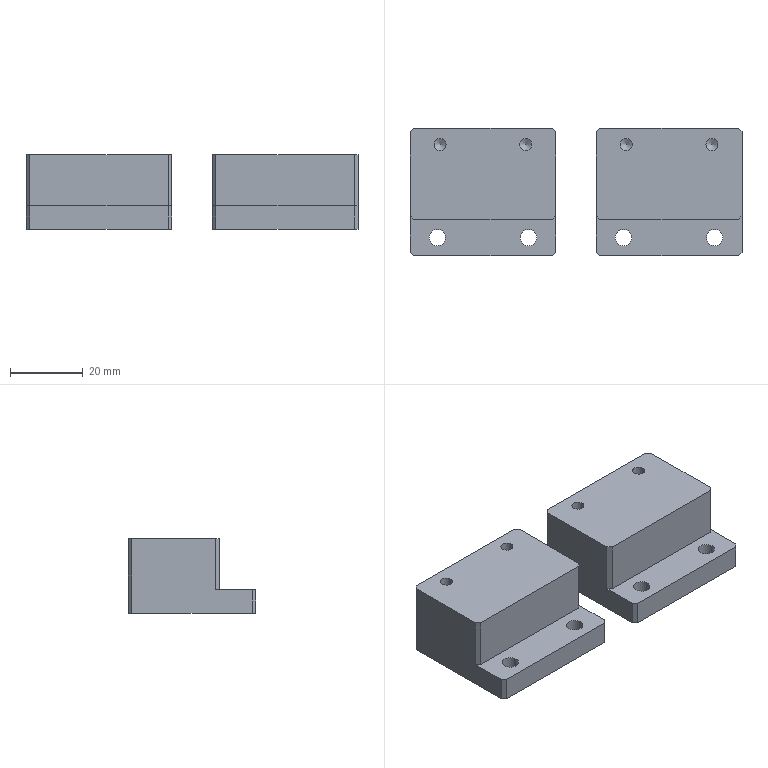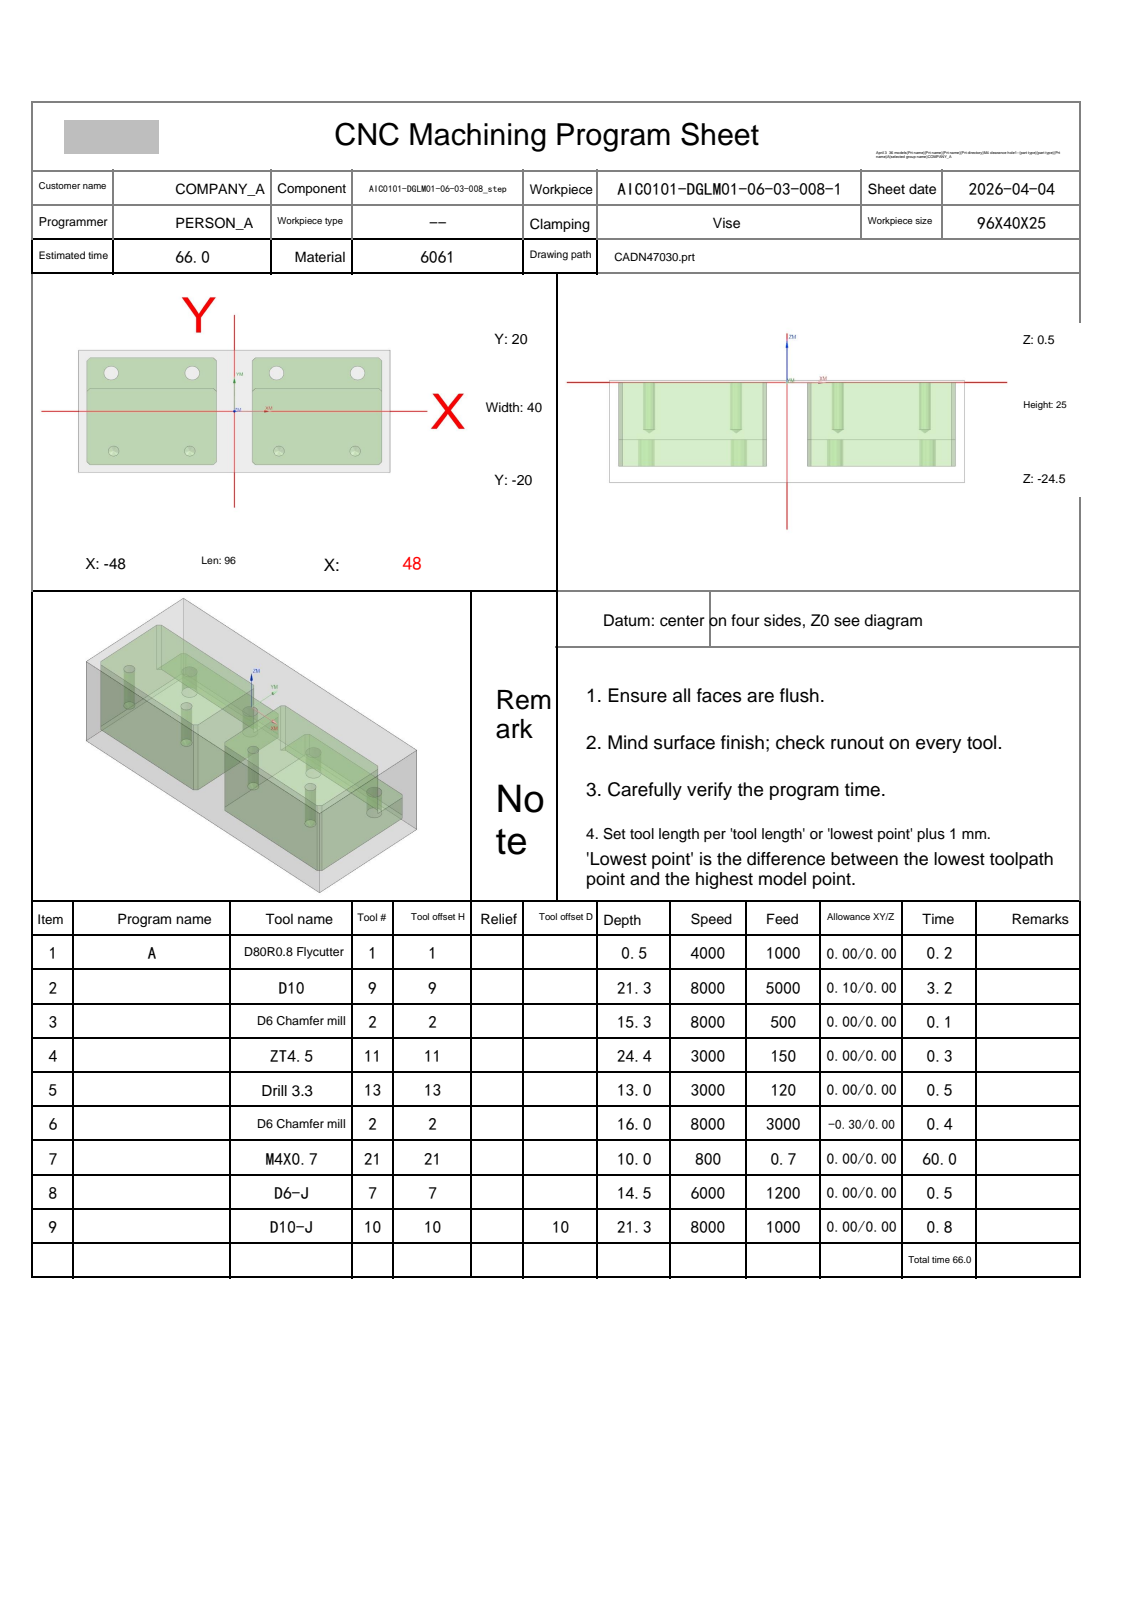NC program | NX | posted by the shop | part box 91 x 35 x 20.5 mm
Lines 1 to 2027 of 2147, first 1232 of 2025 lines:
%
O0001
(Machine time: 121.97 MIN)
(===Total Tool:8===)
(T1=D80R0.8 Flycutter D=80.  R=0.8  D-  H01 Z=-0.   )
(T9=D10     D=10.  R=0.   D-  H09 Z=-20.8 )
(T2=D6 Chamfer mill   D=6.   R=0.   D-  H02 Z=-15.5 )
(T11=ZT4.5  D=4.5  DR_a=118 D-  H11 Z=-23.85)
(T13=Drill 3.3  D=3.3  DR_a=118 D-  H13 Z=-12.49)
(T21=M4X0.7 D=3.3  DR_a=180 D-  H21 Z=-9.5  )
(T7=D6-J    D=6.   R=0.   D7  H07 Z=-14.  )
(T10=D10-J  D=10.  R=0.   D10 H10 Z=-20.8 )
G80 G90 G17 G49 G40
G91 G28 Z0
M01
N1 T01 M06
(D80R0.8 Flycutter  D=80. R=0.8 H=01 ce=0.00 di=0.00)
G00 G90 G54 X90.5 Y0.0 M03 S4000
G43 H01 Z20.
M08
Z2.
G01 Z0.0 F1000.
X85.5
X-85.5
X-90.5
Z2.
G00 Z20.
G91 G28 Z0.0
M05
M09
G91 G28 Z0.0
M01
N2 T09 M06
(D10  D=10. R=0. H=09 ce=0.10 di=0.00)
G00 G90 G54 X25.5 Y-22.6 M03 S8000
G43 H09 Z20.
M08
Z.5
G01 X6.5 Z.417 F5000.
G02 X2.894 Y-21.106 Z.399 I0.0 J5.1
G01 X1.894 Y-20.106 Z.393
G02 X.4 Y-16.5 Z.375 I3.606 J3.606
G01 Y16.5 Z.23
G02 X1.894 Y20.106 Z.213 I5.1 J0.0
G01 X2.894 Y21.106 Z.207
G02 X6.5 Y22.6 Z.189 I3.606 J-3.606
G01 X44.5 Z.022
G02 X48.106 Y21.106 Z.005 I0.0 J-5.1
G01 X49.106 Y20.106 Z-.002
G02 X50.6 Y16.5 Z-.019 I-3.606 J-3.606
G01 Y-16.5 Z-.164
G02 X49.106 Y-20.106 Z-.182 I-5.1 J0.0
G01 X48.106 Y-21.106 Z-.188
G02 X44.5 Y-22.6 Z-.205 I-3.606 J3.606
G01 X6.5 Z-.372
G02 X2.894 Y-21.106 Z-.39 I0.0 J5.1
G01 X1.894 Y-20.106 Z-.396
G02 X.4 Y-16.5 Z-.414 I3.606 J3.606
G01 Y16.5 Z-.559
G02 X1.894 Y20.106 Z-.576 I5.1 J0.0
G01 X2.894 Y21.106 Z-.582
G02 X6.5 Y22.6 Z-.6 I3.606 J-3.606
G01 X44.5 Z-.767
G02 X48.106 Y21.106 Z-.784 I0.0 J-5.1
G01 X49.106 Y20.106 Z-.791
G02 X50.6 Y16.5 Z-.808 I-3.606 J-3.606
G01 Y-16.5 Z-.953
G02 X49.106 Y-20.106 Z-.971 I-5.1 J0.0
G01 X48.106 Y-21.106 Z-.977
G02 X44.5 Y-22.6 Z-.994 I-3.606 J3.606
G01 X6.5 Z-1.161
G02 X2.894 Y-21.106 Z-1.179 I0.0 J5.1
G01 X1.894 Y-20.106 Z-1.185
G02 X.4 Y-16.5 Z-1.203 I3.606 J3.606
G01 Y16.5 Z-1.347
G02 X1.894 Y20.106 Z-1.365 I5.1 J0.0
G01 X2.894 Y21.106 Z-1.371
G02 X6.5 Y22.6 Z-1.389 I3.606 J-3.606
G01 X44.5 Z-1.556
G02 X48.106 Y21.106 Z-1.573 I0.0 J-5.1
G01 X49.106 Y20.106 Z-1.579
G02 X50.6 Y16.5 Z-1.597 I-3.606 J-3.606
G01 Y-16.5 Z-1.742
G02 X49.106 Y-20.106 Z-1.759 I-5.1 J0.0
G01 X48.106 Y-21.106 Z-1.766
G02 X44.5 Y-22.6 Z-1.783 I-3.606 J3.606
G01 X6.5 Z-1.95
G02 X2.894 Y-21.106 Z-1.968 I0.0 J5.1
G01 X1.894 Y-20.106 Z-1.974
G02 X.4 Y-16.5 Z-1.991 I3.606 J3.606
G01 Y16.5 Z-2.136
G02 X1.894 Y20.106 Z-2.154 I5.1 J0.0
G01 X2.894 Y21.106 Z-2.16
G02 X6.5 Y22.6 Z-2.178 I3.606 J-3.606
G01 X44.5 Z-2.345
G02 X48.106 Y21.106 Z-2.362 I0.0 J-5.1
G01 X49.106 Y20.106 Z-2.368
G02 X50.6 Y16.5 Z-2.386 I-3.606 J-3.606
G01 Y-16.5 Z-2.531
G02 X49.106 Y-20.106 Z-2.548 I-5.1 J0.0
G01 X48.106 Y-21.106 Z-2.555
G02 X44.5 Y-22.6 Z-2.572 I-3.606 J3.606
G01 X6.5 Z-2.739
G02 X2.894 Y-21.106 Z-2.757 I0.0 J5.1
G01 X1.894 Y-20.106 Z-2.763
G02 X.4 Y-16.5 Z-2.78 I3.606 J3.606
G01 Y16.5 Z-2.925
G02 X1.894 Y20.106 Z-2.943 I5.1 J0.0
G01 X2.894 Y21.106 Z-2.949
G02 X6.5 Y22.6 Z-2.967 I3.606 J-3.606
G01 X44.5 Z-3.133
G02 X48.106 Y21.106 Z-3.151 I0.0 J-5.1
G01 X49.106 Y20.106 Z-3.157
G02 X50.6 Y16.5 Z-3.175 I-3.606 J-3.606
G01 Y-16.5 Z-3.32
G02 X49.106 Y-20.106 Z-3.337 I-5.1 J0.0
G01 X48.106 Y-21.106 Z-3.343
G02 X44.5 Y-22.6 Z-3.361 I-3.606 J3.606
G01 X6.5 Z-3.528
G02 X2.894 Y-21.106 Z-3.545 I0.0 J5.1
G01 X1.894 Y-20.106 Z-3.552
G02 X.4 Y-16.5 Z-3.569 I3.606 J3.606
G01 Y16.5 Z-3.714
G02 X1.894 Y20.106 Z-3.732 I5.1 J0.0
G01 X2.894 Y21.106 Z-3.738
G02 X6.5 Y22.6 Z-3.755 I3.606 J-3.606
G01 X44.5 Z-3.922
G02 X48.106 Y21.106 Z-3.94 I0.0 J-5.1
G01 X49.106 Y20.106 Z-3.946
G02 X50.6 Y16.5 Z-3.964 I-3.606 J-3.606
G01 Y-16.5 Z-4.109
G02 X49.106 Y-20.106 Z-4.126 I-5.1 J0.0
G01 X48.106 Y-21.106 Z-4.132
G02 X44.5 Y-22.6 Z-4.15 I-3.606 J3.606
G01 X6.5 Z-4.317
G02 X2.894 Y-21.106 Z-4.334 I0.0 J5.1
G01 X1.894 Y-20.106 Z-4.341
G02 X.4 Y-16.5 Z-4.358 I3.606 J3.606
G01 Y16.5 Z-4.503
G02 X1.894 Y20.106 Z-4.521 I5.1 J0.0
G01 X2.894 Y21.106 Z-4.527
G02 X6.5 Y22.6 Z-4.544 I3.606 J-3.606
G01 X44.5 Z-4.711
G02 X48.106 Y21.106 Z-4.729 I0.0 J-5.1
G01 X49.106 Y20.106 Z-4.735
G02 X50.6 Y16.5 Z-4.753 I-3.606 J-3.606
G01 Y-16.5 Z-4.897
G02 X49.106 Y-20.106 Z-4.915 I-5.1 J0.0
G01 X48.106 Y-21.106 Z-4.921
G02 X44.5 Y-22.6 Z-4.939 I-3.606 J3.606
G01 X6.5 Z-5.106
G02 X2.894 Y-21.106 Z-5.123 I0.0 J5.1
G01 X1.894 Y-20.106 Z-5.129
G02 X.4 Y-16.5 Z-5.147 I3.606 J3.606
G01 Y16.5 Z-5.292
G02 X1.894 Y20.106 Z-5.309 I5.1 J0.0
G01 X2.894 Y21.106 Z-5.316
G02 X6.5 Y22.6 Z-5.333 I3.606 J-3.606
G01 X44.5 Z-5.5
G02 X48.106 Y21.106 Z-5.518 I0.0 J-5.1
G01 X49.106 Y20.106 Z-5.524
G02 X50.6 Y16.5 Z-5.541 I-3.606 J-3.606
G01 Y-16.5 Z-5.686
G02 X49.106 Y-20.106 Z-5.704 I-5.1 J0.0
G01 X48.106 Y-21.106 Z-5.71
G02 X44.5 Y-22.6 Z-5.728 I-3.606 J3.606
G01 X6.5 Z-5.895
G02 X2.894 Y-21.106 Z-5.912 I0.0 J5.1
G01 X1.894 Y-20.106 Z-5.918
G02 X.4 Y-16.5 Z-5.936 I3.606 J3.606
G01 Y16.5 Z-6.081
G02 X1.894 Y20.106 Z-6.098 I5.1 J0.0
G01 X2.894 Y21.106 Z-6.105
G02 X6.5 Y22.6 Z-6.122 I3.606 J-3.606
G01 X44.5 Z-6.289
G02 X48.106 Y21.106 Z-6.307 I0.0 J-5.1
G01 X49.106 Y20.106 Z-6.313
G02 X50.6 Y16.5 Z-6.33 I-3.606 J-3.606
G01 Y-16.5 Z-6.475
G02 X49.106 Y-20.106 Z-6.493 I-5.1 J0.0
G01 X48.106 Y-21.106 Z-6.499
G02 X44.5 Y-22.6 Z-6.517 I-3.606 J3.606
G01 X6.5 Z-6.683
G02 X2.894 Y-21.106 Z-6.701 I0.0 J5.1
G01 X1.894 Y-20.106 Z-6.707
G02 X.4 Y-16.5 Z-6.725 I3.606 J3.606
G01 Y16.5 Z-6.87
G02 X1.894 Y20.106 Z-6.887 I5.1 J0.0
G01 X2.894 Y21.106 Z-6.893
G02 X6.5 Y22.6 Z-6.911 I3.606 J-3.606
G01 X44.5 Z-7.078
G02 X48.106 Y21.106 Z-7.095 I0.0 J-5.1
G01 X49.106 Y20.106 Z-7.102
G02 X50.6 Y16.5 Z-7.119 I-3.606 J-3.606
G01 Y-16.5 Z-7.264
G02 X49.106 Y-20.106 Z-7.282 I-5.1 J0.0
G01 X48.106 Y-21.106 Z-7.288
G02 X44.5 Y-22.6 Z-7.305 I-3.606 J3.606
G01 X6.5 Z-7.472
G02 X2.894 Y-21.106 Z-7.49 I0.0 J5.1
G01 X1.894 Y-20.106 Z-7.496
G02 X.4 Y-16.5 Z-7.514 I3.606 J3.606
G01 Y16.5 Z-7.659
G02 X1.894 Y20.106 Z-7.676 I5.1 J0.0
G01 X2.894 Y21.106 Z-7.682
G02 X6.5 Y22.6 Z-7.7 I3.606 J-3.606
G01 X44.5 Z-7.867
G02 X48.106 Y21.106 Z-7.884 I0.0 J-5.1
G01 X49.106 Y20.106 Z-7.891
G02 X50.6 Y16.5 Z-7.908 I-3.606 J-3.606
G01 Y-16.5 Z-8.053
G02 X49.106 Y-20.106 Z-8.071 I-5.1 J0.0
G01 X48.106 Y-21.106 Z-8.077
G02 X44.5 Y-22.6 Z-8.094 I-3.606 J3.606
G01 X6.5 Z-8.261
G02 X2.894 Y-21.106 Z-8.279 I0.0 J5.1
G01 X1.894 Y-20.106 Z-8.285
G02 X.4 Y-16.5 Z-8.303 I3.606 J3.606
G01 Y16.5 Z-8.447
G02 X1.894 Y20.106 Z-8.465 I5.1 J0.0
G01 X2.894 Y21.106 Z-8.471
G02 X6.5 Y22.6 Z-8.489 I3.606 J-3.606
G01 X44.5 Z-8.656
G02 X48.106 Y21.106 Z-8.673 I0.0 J-5.1
G01 X49.106 Y20.106 Z-8.679
G02 X50.6 Y16.5 Z-8.697 I-3.606 J-3.606
G01 Y-16.5 Z-8.842
G02 X49.106 Y-20.106 Z-8.859 I-5.1 J0.0
G01 X48.106 Y-21.106 Z-8.866
G02 X44.5 Y-22.6 Z-8.883 I-3.606 J3.606
G01 X6.5 Z-9.05
G02 X2.894 Y-21.106 Z-9.068 I0.0 J5.1
G01 X1.894 Y-20.106 Z-9.074
G02 X.4 Y-16.5 Z-9.091 I3.606 J3.606
G01 Y16.5 Z-9.236
G02 X1.894 Y20.106 Z-9.254 I5.1 J0.0
G01 X2.894 Y21.106 Z-9.26
G02 X6.5 Y22.6 Z-9.278 I3.606 J-3.606
G01 X44.5 Z-9.445
G02 X48.106 Y21.106 Z-9.462 I0.0 J-5.1
G01 X49.106 Y20.106 Z-9.468
G02 X50.6 Y16.5 Z-9.486 I-3.606 J-3.606
G01 Y-16.5 Z-9.631
G02 X49.106 Y-20.106 Z-9.648 I-5.1 J0.0
G01 X48.106 Y-21.106 Z-9.655
G02 X44.5 Y-22.6 Z-9.672 I-3.606 J3.606
G01 X6.5 Z-9.839
G02 X2.894 Y-21.106 Z-9.857 I0.0 J5.1
G01 X1.894 Y-20.106 Z-9.863
G02 X.4 Y-16.5 Z-9.88 I3.606 J3.606
G01 Y16.5 Z-10.025
G02 X1.894 Y20.106 Z-10.043 I5.1 J0.0
G01 X2.894 Y21.106 Z-10.049
G02 X6.5 Y22.6 Z-10.067 I3.606 J-3.606
G01 X44.5 Z-10.233
G02 X48.106 Y21.106 Z-10.251 I0.0 J-5.1
G01 X49.106 Y20.106 Z-10.257
G02 X50.6 Y16.5 Z-10.275 I-3.606 J-3.606
G01 Y-16.5 Z-10.42
G02 X49.106 Y-20.106 Z-10.437 I-5.1 J0.0
G01 X48.106 Y-21.106 Z-10.443
G02 X44.5 Y-22.6 Z-10.461 I-3.606 J3.606
G01 X6.5 Z-10.628
G02 X2.894 Y-21.106 Z-10.645 I0.0 J5.1
G01 X1.894 Y-20.106 Z-10.652
G02 X.4 Y-16.5 Z-10.669 I3.606 J3.606
G01 Y16.5 Z-10.814
G02 X1.894 Y20.106 Z-10.832 I5.1 J0.0
G01 X2.894 Y21.106 Z-10.838
G02 X6.5 Y22.6 Z-10.855 I3.606 J-3.606
G01 X44.5 Z-11.022
G02 X48.106 Y21.106 Z-11.04 I0.0 J-5.1
G01 X49.106 Y20.106 Z-11.046
G02 X50.6 Y16.5 Z-11.064 I-3.606 J-3.606
G01 Y-16.5 Z-11.209
G02 X49.106 Y-20.106 Z-11.226 I-5.1 J0.0
G01 X48.106 Y-21.106 Z-11.232
G02 X44.5 Y-22.6 Z-11.25 I-3.606 J3.606
G01 X6.5 Z-11.417
G02 X2.894 Y-21.106 Z-11.434 I0.0 J5.1
G01 X1.894 Y-20.106 Z-11.441
G02 X.4 Y-16.5 Z-11.458 I3.606 J3.606
G01 Y16.5 Z-11.603
G02 X1.894 Y20.106 Z-11.621 I5.1 J0.0
G01 X2.894 Y21.106 Z-11.627
G02 X6.5 Y22.6 Z-11.644 I3.606 J-3.606
G01 X44.5 Z-11.811
G02 X48.106 Y21.106 Z-11.829 I0.0 J-5.1
G01 X49.106 Y20.106 Z-11.835
G02 X50.6 Y16.5 Z-11.853 I-3.606 J-3.606
G01 Y-16.5 Z-11.997
G02 X49.106 Y-20.106 Z-12.015 I-5.1 J0.0
G01 X48.106 Y-21.106 Z-12.021
G02 X44.5 Y-22.6 Z-12.039 I-3.606 J3.606
G01 X6.5 Z-12.206
G02 X2.894 Y-21.106 Z-12.223 I0.0 J5.1
G01 X1.894 Y-20.106 Z-12.229
G02 X.4 Y-16.5 Z-12.247 I3.606 J3.606
G01 Y16.5 Z-12.392
G02 X1.894 Y20.106 Z-12.409 I5.1 J0.0
G01 X2.894 Y21.106 Z-12.416
G02 X6.5 Y22.6 Z-12.433 I3.606 J-3.606
G01 X44.5 Z-12.6
G02 X48.106 Y21.106 Z-12.618 I0.0 J-5.1
G01 X49.106 Y20.106 Z-12.624
G02 X50.6 Y16.5 Z-12.641 I-3.606 J-3.606
G01 Y-16.5 Z-12.786
G02 X49.106 Y-20.106 Z-12.804 I-5.1 J0.0
G01 X48.106 Y-21.106 Z-12.81
G02 X44.5 Y-22.6 Z-12.828 I-3.606 J3.606
G01 X6.5 Z-12.995
G02 X2.894 Y-21.106 Z-13.012 I0.0 J5.1
G01 X1.894 Y-20.106 Z-13.018
G02 X.4 Y-16.5 Z-13.036 I3.606 J3.606
G01 Y16.5 Z-13.181
G02 X1.894 Y20.106 Z-13.198 I5.1 J0.0
G01 X2.894 Y21.106 Z-13.205
G02 X6.5 Y22.6 Z-13.222 I3.606 J-3.606
G01 X44.5 Z-13.389
G02 X48.106 Y21.106 Z-13.407 I0.0 J-5.1
G01 X49.106 Y20.106 Z-13.413
G02 X50.6 Y16.5 Z-13.43 I-3.606 J-3.606
G01 Y-16.5 Z-13.575
G02 X49.106 Y-20.106 Z-13.593 I-5.1 J0.0
G01 X48.106 Y-21.106 Z-13.599
G02 X44.5 Y-22.6 Z-13.617 I-3.606 J3.606
G01 X6.5 Z-13.783
G02 X2.894 Y-21.106 Z-13.801 I0.0 J5.1
G01 X1.894 Y-20.106 Z-13.807
G02 X.4 Y-16.5 Z-13.825 I3.606 J3.606
G01 Y16.5 Z-13.97
G02 X1.894 Y20.106 Z-13.987 I5.1 J0.0
G01 X2.894 Y21.106 Z-13.993
G02 X6.5 Y22.6 Z-14.011 I3.606 J-3.606
G01 X44.5 Z-14.178
G02 X48.106 Y21.106 Z-14.195 I0.0 J-5.1
G01 X49.106 Y20.106 Z-14.202
G02 X50.6 Y16.5 Z-14.219 I-3.606 J-3.606
G01 Y-16.5 Z-14.364
G02 X49.106 Y-20.106 Z-14.382 I-5.1 J0.0
G01 X48.106 Y-21.106 Z-14.388
G02 X44.5 Y-22.6 Z-14.405 I-3.606 J3.606
G01 X6.5 Z-14.572
G02 X2.894 Y-21.106 Z-14.59 I0.0 J5.1
G01 X1.894 Y-20.106 Z-14.596
G02 X.4 Y-16.5 Z-14.614 I3.606 J3.606
G01 Y16.5 Z-14.759
G02 X1.894 Y20.106 Z-14.776 I5.1 J0.0
G01 X2.894 Y21.106 Z-14.782
G02 X6.5 Y22.6 Z-14.8 I3.606 J-3.606
G01 X44.5 Z-14.967
G02 X48.106 Y21.106 Z-14.984 I0.0 J-5.1
G01 X49.106 Y20.106 Z-14.991
G02 X50.6 Y16.5 Z-15.008 I-3.606 J-3.606
G01 Y-16.5 Z-15.153
G02 X49.106 Y-20.106 Z-15.171 I-5.1 J0.0
G01 X48.106 Y-21.106 Z-15.177
G02 X44.5 Y-22.6 Z-15.194 I-3.606 J3.606
G01 X6.5 Z-15.361
G02 X2.894 Y-21.106 Z-15.379 I0.0 J5.1
G01 X1.894 Y-20.106 Z-15.385
G02 X.4 Y-16.5 Z-15.403 I3.606 J3.606
G01 Y16.5 Z-15.547
G02 X1.894 Y20.106 Z-15.565 I5.1 J0.0
G01 X2.894 Y21.106 Z-15.571
G02 X6.5 Y22.6 Z-15.589 I3.606 J-3.606
G01 X44.5 Z-15.756
G02 X48.106 Y21.106 Z-15.773 I0.0 J-5.1
G01 X49.106 Y20.106 Z-15.779
G02 X50.6 Y16.5 Z-15.797 I-3.606 J-3.606
G01 Y-16.5 Z-15.942
G02 X49.106 Y-20.106 Z-15.959 I-5.1 J0.0
G01 X48.106 Y-21.106 Z-15.966
G02 X44.5 Y-22.6 Z-15.983 I-3.606 J3.606
G01 X6.5 Z-16.15
G02 X2.894 Y-21.106 Z-16.168 I0.0 J5.1
G01 X1.894 Y-20.106 Z-16.174
G02 X.4 Y-16.5 Z-16.191 I3.606 J3.606
G01 Y16.5 Z-16.336
G02 X1.894 Y20.106 Z-16.354 I5.1 J0.0
G01 X2.894 Y21.106 Z-16.36
G02 X6.5 Y22.6 Z-16.378 I3.606 J-3.606
G01 X44.5 Z-16.545
G02 X48.106 Y21.106 Z-16.562 I0.0 J-5.1
G01 X49.106 Y20.106 Z-16.568
G02 X50.6 Y16.5 Z-16.586 I-3.606 J-3.606
G01 Y-16.5 Z-16.731
G02 X49.106 Y-20.106 Z-16.748 I-5.1 J0.0
G01 X48.106 Y-21.106 Z-16.755
G02 X44.5 Y-22.6 Z-16.772 I-3.606 J3.606
G01 X6.5 Z-16.939
G02 X2.894 Y-21.106 Z-16.957 I0.0 J5.1
G01 X1.894 Y-20.106 Z-16.963
G02 X.4 Y-16.5 Z-16.98 I3.606 J3.606
G01 Y16.5 Z-17.125
G02 X1.894 Y20.106 Z-17.143 I5.1 J0.0
G01 X2.894 Y21.106 Z-17.149
G02 X6.5 Y22.6 Z-17.167 I3.606 J-3.606
G01 X44.5 Z-17.333
G02 X48.106 Y21.106 Z-17.351 I0.0 J-5.1
G01 X49.106 Y20.106 Z-17.357
G02 X50.6 Y16.5 Z-17.375 I-3.606 J-3.606
G01 Y-16.5 Z-17.52
G02 X49.106 Y-20.106 Z-17.537 I-5.1 J0.0
G01 X48.106 Y-21.106 Z-17.543
G02 X44.5 Y-22.6 Z-17.561 I-3.606 J3.606
G01 X6.5 Z-17.728
G02 X2.894 Y-21.106 Z-17.745 I0.0 J5.1
G01 X1.894 Y-20.106 Z-17.752
G02 X.4 Y-16.5 Z-17.769 I3.606 J3.606
G01 Y16.5 Z-17.914
G02 X1.894 Y20.106 Z-17.932 I5.1 J0.0
G01 X2.894 Y21.106 Z-17.938
G02 X6.5 Y22.6 Z-17.955 I3.606 J-3.606
G01 X44.5 Z-18.122
G02 X48.106 Y21.106 Z-18.14 I0.0 J-5.1
G01 X49.106 Y20.106 Z-18.146
G02 X50.6 Y16.5 Z-18.164 I-3.606 J-3.606
G01 Y-16.5 Z-18.309
G02 X49.106 Y-20.106 Z-18.326 I-5.1 J0.0
G01 X48.106 Y-21.106 Z-18.332
G02 X44.5 Y-22.6 Z-18.35 I-3.606 J3.606
G01 X6.5 Z-18.517
G02 X2.894 Y-21.106 Z-18.534 I0.0 J5.1
G01 X1.894 Y-20.106 Z-18.541
G02 X.4 Y-16.5 Z-18.558 I3.606 J3.606
G01 Y16.5 Z-18.703
G02 X1.894 Y20.106 Z-18.721 I5.1 J0.0
G01 X2.894 Y21.106 Z-18.727
G02 X6.5 Y22.6 Z-18.744 I3.606 J-3.606
G01 X44.5 Z-18.911
G02 X48.106 Y21.106 Z-18.929 I0.0 J-5.1
G01 X49.106 Y20.106 Z-18.935
G02 X50.6 Y16.5 Z-18.953 I-3.606 J-3.606
G01 Y-16.5 Z-19.097
G02 X49.106 Y-20.106 Z-19.115 I-5.1 J0.0
G01 X48.106 Y-21.106 Z-19.121
G02 X44.5 Y-22.6 Z-19.139 I-3.606 J3.606
G01 X6.5 Z-19.306
G02 X2.894 Y-21.106 Z-19.323 I0.0 J5.1
G01 X1.894 Y-20.106 Z-19.329
G02 X.4 Y-16.5 Z-19.347 I3.606 J3.606
G01 Y16.5 Z-19.492
G02 X1.894 Y20.106 Z-19.509 I5.1 J0.0
G01 X2.894 Y21.106 Z-19.516
G02 X6.5 Y22.6 Z-19.533 I3.606 J-3.606
G01 X44.5 Z-19.7
G02 X48.106 Y21.106 Z-19.718 I0.0 J-5.1
G01 X49.106 Y20.106 Z-19.724
G02 X50.6 Y16.5 Z-19.741 I-3.606 J-3.606
G01 Y-16.5 Z-19.886
G02 X49.106 Y-20.106 Z-19.904 I-5.1 J0.0
G01 X48.106 Y-21.106 Z-19.91
G02 X44.5 Y-22.6 Z-19.928 I-3.606 J3.606
G01 X6.5 Z-20.095
G02 X2.894 Y-21.106 Z-20.112 I0.0 J5.1
G01 X1.894 Y-20.106 Z-20.118
G02 X.4 Y-16.5 Z-20.136 I3.606 J3.606
G01 Y16.5 Z-20.281
G02 X1.894 Y20.106 Z-20.298 I5.1 J0.0
G01 X2.894 Y21.106 Z-20.305
G02 X6.5 Y22.6 Z-20.322 I3.606 J-3.606
G01 X44.5 Z-20.489
G02 X48.106 Y21.106 Z-20.507 I0.0 J-5.1
G01 X49.106 Y20.106 Z-20.513
G02 X50.6 Y16.5 Z-20.53 I-3.606 J-3.606
G01 Y-16.5 Z-20.675
G02 X49.106 Y-20.106 Z-20.693 I-5.1 J0.0
G01 X48.106 Y-21.106 Z-20.699
G02 X44.5 Y-22.6 Z-20.717 I-3.606 J3.606
G01 X25.5 Z-20.8
X6.5
G02 X2.894 Y-21.106 I0.0 J5.1
G01 X1.894 Y-20.106
G02 X.4 Y-16.5 I3.606 J3.606
G01 Y16.5
G02 X1.894 Y20.106 I5.1 J0.0
G01 X2.894 Y21.106
G02 X6.5 Y22.6 I3.606 J-3.606
G01 X44.5
G02 X48.106 Y21.106 I0.0 J-5.1
G01 X49.106 Y20.106
G02 X50.6 Y16.5 I-3.606 J-3.606
G01 Y-16.5
G02 X49.106 Y-20.106 I-5.1 J0.0
G01 X48.106 Y-21.106
G02 X44.5 Y-22.6 I-3.606 J3.606
G01 X25.5
X25.
Z-19.8
G00 Z20.
X-25.5
Z.5
G01 X-44.5 Z.417
G02 X-48.106 Y-21.106 Z.399 I0.0 J5.1
G01 X-49.106 Y-20.106 Z.393
G02 X-50.6 Y-16.5 Z.375 I3.606 J3.606
G01 Y16.5 Z.23
G02 X-49.106 Y20.106 Z.213 I5.1 J0.0
G01 X-48.106 Y21.106 Z.207
G02 X-44.5 Y22.6 Z.189 I3.606 J-3.606
G01 X-6.5 Z.022
G02 X-2.894 Y21.106 Z.005 I0.0 J-5.1
G01 X-1.894 Y20.106 Z-.002
G02 X-.4 Y16.5 Z-.019 I-3.606 J-3.606
G01 Y-16.5 Z-.164
G02 X-1.894 Y-20.106 Z-.182 I-5.1 J0.0
G01 X-2.894 Y-21.106 Z-.188
G02 X-6.5 Y-22.6 Z-.205 I-3.606 J3.606
G01 X-44.5 Z-.372
G02 X-48.106 Y-21.106 Z-.39 I0.0 J5.1
G01 X-49.106 Y-20.106 Z-.396
G02 X-50.6 Y-16.5 Z-.414 I3.606 J3.606
G01 Y16.5 Z-.559
G02 X-49.106 Y20.106 Z-.576 I5.1 J0.0
G01 X-48.106 Y21.106 Z-.582
G02 X-44.5 Y22.6 Z-.6 I3.606 J-3.606
G01 X-6.5 Z-.767
G02 X-2.894 Y21.106 Z-.784 I0.0 J-5.1
G01 X-1.894 Y20.106 Z-.791
G02 X-.4 Y16.5 Z-.808 I-3.606 J-3.606
G01 Y-16.5 Z-.953
G02 X-1.894 Y-20.106 Z-.971 I-5.1 J0.0
G01 X-2.894 Y-21.106 Z-.977
G02 X-6.5 Y-22.6 Z-.994 I-3.606 J3.606
G01 X-44.5 Z-1.161
G02 X-48.106 Y-21.106 Z-1.179 I0.0 J5.1
G01 X-49.106 Y-20.106 Z-1.185
G02 X-50.6 Y-16.5 Z-1.203 I3.606 J3.606
G01 Y16.5 Z-1.347
G02 X-49.106 Y20.106 Z-1.365 I5.1 J0.0
G01 X-48.106 Y21.106 Z-1.371
G02 X-44.5 Y22.6 Z-1.389 I3.606 J-3.606
G01 X-6.5 Z-1.556
G02 X-2.894 Y21.106 Z-1.573 I0.0 J-5.1
G01 X-1.894 Y20.106 Z-1.579
G02 X-.4 Y16.5 Z-1.597 I-3.606 J-3.606
G01 Y-16.5 Z-1.742
G02 X-1.894 Y-20.106 Z-1.759 I-5.1 J0.0
G01 X-2.894 Y-21.106 Z-1.766
G02 X-6.5 Y-22.6 Z-1.783 I-3.606 J3.606
G01 X-44.5 Z-1.95
G02 X-48.106 Y-21.106 Z-1.968 I0.0 J5.1
G01 X-49.106 Y-20.106 Z-1.974
G02 X-50.6 Y-16.5 Z-1.991 I3.606 J3.606
G01 Y16.5 Z-2.136
G02 X-49.106 Y20.106 Z-2.154 I5.1 J0.0
G01 X-48.106 Y21.106 Z-2.16
G02 X-44.5 Y22.6 Z-2.178 I3.606 J-3.606
G01 X-6.5 Z-2.345
G02 X-2.894 Y21.106 Z-2.362 I0.0 J-5.1
G01 X-1.894 Y20.106 Z-2.368
G02 X-.4 Y16.5 Z-2.386 I-3.606 J-3.606
G01 Y-16.5 Z-2.531
G02 X-1.894 Y-20.106 Z-2.548 I-5.1 J0.0
G01 X-2.894 Y-21.106 Z-2.555
G02 X-6.5 Y-22.6 Z-2.572 I-3.606 J3.606
G01 X-44.5 Z-2.739
G02 X-48.106 Y-21.106 Z-2.757 I0.0 J5.1
G01 X-49.106 Y-20.106 Z-2.763
G02 X-50.6 Y-16.5 Z-2.78 I3.606 J3.606
G01 Y16.5 Z-2.925
G02 X-49.106 Y20.106 Z-2.943 I5.1 J0.0
G01 X-48.106 Y21.106 Z-2.949
G02 X-44.5 Y22.6 Z-2.967 I3.606 J-3.606
G01 X-6.5 Z-3.133
G02 X-2.894 Y21.106 Z-3.151 I0.0 J-5.1
G01 X-1.894 Y20.106 Z-3.157
G02 X-.4 Y16.5 Z-3.175 I-3.606 J-3.606
G01 Y-16.5 Z-3.32
G02 X-1.894 Y-20.106 Z-3.337 I-5.1 J0.0
G01 X-2.894 Y-21.106 Z-3.343
G02 X-6.5 Y-22.6 Z-3.361 I-3.606 J3.606
G01 X-44.5 Z-3.528
G02 X-48.106 Y-21.106 Z-3.545 I0.0 J5.1
G01 X-49.106 Y-20.106 Z-3.552
G02 X-50.6 Y-16.5 Z-3.569 I3.606 J3.606
G01 Y16.5 Z-3.714
G02 X-49.106 Y20.106 Z-3.732 I5.1 J0.0
G01 X-48.106 Y21.106 Z-3.738
G02 X-44.5 Y22.6 Z-3.755 I3.606 J-3.606
G01 X-6.5 Z-3.922
G02 X-2.894 Y21.106 Z-3.94 I0.0 J-5.1
G01 X-1.894 Y20.106 Z-3.946
G02 X-.4 Y16.5 Z-3.964 I-3.606 J-3.606
G01 Y-16.5 Z-4.109
G02 X-1.894 Y-20.106 Z-4.126 I-5.1 J0.0
G01 X-2.894 Y-21.106 Z-4.132
G02 X-6.5 Y-22.6 Z-4.15 I-3.606 J3.606
G01 X-44.5 Z-4.317
G02 X-48.106 Y-21.106 Z-4.334 I0.0 J5.1
G01 X-49.106 Y-20.106 Z-4.341
G02 X-50.6 Y-16.5 Z-4.358 I3.606 J3.606
G01 Y16.5 Z-4.503
G02 X-49.106 Y20.106 Z-4.521 I5.1 J0.0
G01 X-48.106 Y21.106 Z-4.527
G02 X-44.5 Y22.6 Z-4.544 I3.606 J-3.606
G01 X-6.5 Z-4.711
G02 X-2.894 Y21.106 Z-4.729 I0.0 J-5.1
G01 X-1.894 Y20.106 Z-4.735
G02 X-.4 Y16.5 Z-4.753 I-3.606 J-3.606
G01 Y-16.5 Z-4.897
G02 X-1.894 Y-20.106 Z-4.915 I-5.1 J0.0
G01 X-2.894 Y-21.106 Z-4.921
G02 X-6.5 Y-22.6 Z-4.939 I-3.606 J3.606
G01 X-44.5 Z-5.106
G02 X-48.106 Y-21.106 Z-5.123 I0.0 J5.1
G01 X-49.106 Y-20.106 Z-5.129
G02 X-50.6 Y-16.5 Z-5.147 I3.606 J3.606
G01 Y16.5 Z-5.292
G02 X-49.106 Y20.106 Z-5.309 I5.1 J0.0
G01 X-48.106 Y21.106 Z-5.316
G02 X-44.5 Y22.6 Z-5.333 I3.606 J-3.606
G01 X-6.5 Z-5.5
G02 X-2.894 Y21.106 Z-5.518 I0.0 J-5.1
G01 X-1.894 Y20.106 Z-5.524
G02 X-.4 Y16.5 Z-5.541 I-3.606 J-3.606
G01 Y-16.5 Z-5.686
G02 X-1.894 Y-20.106 Z-5.704 I-5.1 J0.0
G01 X-2.894 Y-21.106 Z-5.71
G02 X-6.5 Y-22.6 Z-5.728 I-3.606 J3.606
G01 X-44.5 Z-5.895
G02 X-48.106 Y-21.106 Z-5.912 I0.0 J5.1
G01 X-49.106 Y-20.106 Z-5.918
G02 X-50.6 Y-16.5 Z-5.936 I3.606 J3.606
G01 Y16.5 Z-6.081
G02 X-49.106 Y20.106 Z-6.098 I5.1 J0.0
G01 X-48.106 Y21.106 Z-6.105
G02 X-44.5 Y22.6 Z-6.122 I3.606 J-3.606
G01 X-6.5 Z-6.289
G02 X-2.894 Y21.106 Z-6.307 I0.0 J-5.1
G01 X-1.894 Y20.106 Z-6.313
G02 X-.4 Y16.5 Z-6.33 I-3.606 J-3.606
G01 Y-16.5 Z-6.475
G02 X-1.894 Y-20.106 Z-6.493 I-5.1 J0.0
G01 X-2.894 Y-21.106 Z-6.499
G02 X-6.5 Y-22.6 Z-6.517 I-3.606 J3.606
G01 X-44.5 Z-6.683
G02 X-48.106 Y-21.106 Z-6.701 I0.0 J5.1
G01 X-49.106 Y-20.106 Z-6.707
G02 X-50.6 Y-16.5 Z-6.725 I3.606 J3.606
G01 Y16.5 Z-6.87
G02 X-49.106 Y20.106 Z-6.887 I5.1 J0.0
G01 X-48.106 Y21.106 Z-6.893
G02 X-44.5 Y22.6 Z-6.911 I3.606 J-3.606
G01 X-6.5 Z-7.078
G02 X-2.894 Y21.106 Z-7.095 I0.0 J-5.1
G01 X-1.894 Y20.106 Z-7.102
G02 X-.4 Y16.5 Z-7.119 I-3.606 J-3.606
G01 Y-16.5 Z-7.264
G02 X-1.894 Y-20.106 Z-7.282 I-5.1 J0.0
G01 X-2.894 Y-21.106 Z-7.288
G02 X-6.5 Y-22.6 Z-7.305 I-3.606 J3.606
G01 X-44.5 Z-7.472
G02 X-48.106 Y-21.106 Z-7.49 I0.0 J5.1
G01 X-49.106 Y-20.106 Z-7.496
G02 X-50.6 Y-16.5 Z-7.514 I3.606 J3.606
G01 Y16.5 Z-7.659
G02 X-49.106 Y20.106 Z-7.676 I5.1 J0.0
G01 X-48.106 Y21.106 Z-7.682
G02 X-44.5 Y22.6 Z-7.7 I3.606 J-3.606
G01 X-6.5 Z-7.867
G02 X-2.894 Y21.106 Z-7.884 I0.0 J-5.1
G01 X-1.894 Y20.106 Z-7.891
G02 X-.4 Y16.5 Z-7.908 I-3.606 J-3.606
G01 Y-16.5 Z-8.053
G02 X-1.894 Y-20.106 Z-8.071 I-5.1 J0.0
G01 X-2.894 Y-21.106 Z-8.077
G02 X-6.5 Y-22.6 Z-8.094 I-3.606 J3.606
G01 X-44.5 Z-8.261
G02 X-48.106 Y-21.106 Z-8.279 I0.0 J5.1
G01 X-49.106 Y-20.106 Z-8.285
G02 X-50.6 Y-16.5 Z-8.303 I3.606 J3.606
G01 Y16.5 Z-8.447
G02 X-49.106 Y20.106 Z-8.465 I5.1 J0.0
G01 X-48.106 Y21.106 Z-8.471
G02 X-44.5 Y22.6 Z-8.489 I3.606 J-3.606
G01 X-6.5 Z-8.656
G02 X-2.894 Y21.106 Z-8.673 I0.0 J-5.1
G01 X-1.894 Y20.106 Z-8.679
G02 X-.4 Y16.5 Z-8.697 I-3.606 J-3.606
G01 Y-16.5 Z-8.842
G02 X-1.894 Y-20.106 Z-8.859 I-5.1 J0.0
G01 X-2.894 Y-21.106 Z-8.866
G02 X-6.5 Y-22.6 Z-8.883 I-3.606 J3.606
G01 X-44.5 Z-9.05
G02 X-48.106 Y-21.106 Z-9.068 I0.0 J5.1
G01 X-49.106 Y-20.106 Z-9.074
G02 X-50.6 Y-16.5 Z-9.091 I3.606 J3.606
G01 Y16.5 Z-9.236
G02 X-49.106 Y20.106 Z-9.254 I5.1 J0.0
G01 X-48.106 Y21.106 Z-9.26
G02 X-44.5 Y22.6 Z-9.278 I3.606 J-3.606
G01 X-6.5 Z-9.445
G02 X-2.894 Y21.106 Z-9.462 I0.0 J-5.1
G01 X-1.894 Y20.106 Z-9.468
G02 X-.4 Y16.5 Z-9.486 I-3.606 J-3.606
G01 Y-16.5 Z-9.631
G02 X-1.894 Y-20.106 Z-9.648 I-5.1 J0.0
G01 X-2.894 Y-21.106 Z-9.655
G02 X-6.5 Y-22.6 Z-9.672 I-3.606 J3.606
G01 X-44.5 Z-9.839
G02 X-48.106 Y-21.106 Z-9.857 I0.0 J5.1
G01 X-49.106 Y-20.106 Z-9.863
G02 X-50.6 Y-16.5 Z-9.88 I3.606 J3.606
G01 Y16.5 Z-10.025
G02 X-49.106 Y20.106 Z-10.043 I5.1 J0.0
G01 X-48.106 Y21.106 Z-10.049
G02 X-44.5 Y22.6 Z-10.067 I3.606 J-3.606
G01 X-6.5 Z-10.233
G02 X-2.894 Y21.106 Z-10.251 I0.0 J-5.1
G01 X-1.894 Y20.106 Z-10.257
G02 X-.4 Y16.5 Z-10.275 I-3.606 J-3.606
G01 Y-16.5 Z-10.42
G02 X-1.894 Y-20.106 Z-10.437 I-5.1 J0.0
G01 X-2.894 Y-21.106 Z-10.443
G02 X-6.5 Y-22.6 Z-10.461 I-3.606 J3.606
G01 X-44.5 Z-10.628
G02 X-48.106 Y-21.106 Z-10.645 I0.0 J5.1
G01 X-49.106 Y-20.106 Z-10.652
G02 X-50.6 Y-16.5 Z-10.669 I3.606 J3.606
G01 Y16.5 Z-10.814
G02 X-49.106 Y20.106 Z-10.832 I5.1 J0.0
G01 X-48.106 Y21.106 Z-10.838
G02 X-44.5 Y22.6 Z-10.855 I3.606 J-3.606
G01 X-6.5 Z-11.022
G02 X-2.894 Y21.106 Z-11.04 I0.0 J-5.1
G01 X-1.894 Y20.106 Z-11.046
G02 X-.4 Y16.5 Z-11.064 I-3.606 J-3.606
G01 Y-16.5 Z-11.209
G02 X-1.894 Y-20.106 Z-11.226 I-5.1 J0.0
G01 X-2.894 Y-21.106 Z-11.232
G02 X-6.5 Y-22.6 Z-11.25 I-3.606 J3.606
G01 X-44.5 Z-11.417
G02 X-48.106 Y-21.106 Z-11.434 I0.0 J5.1
G01 X-49.106 Y-20.106 Z-11.441
G02 X-50.6 Y-16.5 Z-11.458 I3.606 J3.606
G01 Y16.5 Z-11.603
G02 X-49.106 Y20.106 Z-11.621 I5.1 J0.0
G01 X-48.106 Y21.106 Z-11.627
G02 X-44.5 Y22.6 Z-11.644 I3.606 J-3.606
G01 X-6.5 Z-11.811
G02 X-2.894 Y21.106 Z-11.829 I0.0 J-5.1
G01 X-1.894 Y20.106 Z-11.835
G02 X-.4 Y16.5 Z-11.853 I-3.606 J-3.606
G01 Y-16.5 Z-11.997
G02 X-1.894 Y-20.106 Z-12.015 I-5.1 J0.0
G01 X-2.894 Y-21.106 Z-12.021
G02 X-6.5 Y-22.6 Z-12.039 I-3.606 J3.606
G01 X-44.5 Z-12.206
G02 X-48.106 Y-21.106 Z-12.223 I0.0 J5.1
G01 X-49.106 Y-20.106 Z-12.229
G02 X-50.6 Y-16.5 Z-12.247 I3.606 J3.606
G01 Y16.5 Z-12.392
G02 X-49.106 Y20.106 Z-12.409 I5.1 J0.0
G01 X-48.106 Y21.106 Z-12.416
G02 X-44.5 Y22.6 Z-12.433 I3.606 J-3.606
G01 X-6.5 Z-12.6
G02 X-2.894 Y21.106 Z-12.618 I0.0 J-5.1
G01 X-1.894 Y20.106 Z-12.624
G02 X-.4 Y16.5 Z-12.641 I-3.606 J-3.606
G01 Y-16.5 Z-12.786
G02 X-1.894 Y-20.106 Z-12.804 I-5.1 J0.0
G01 X-2.894 Y-21.106 Z-12.81
G02 X-6.5 Y-22.6 Z-12.828 I-3.606 J3.606
G01 X-44.5 Z-12.995
G02 X-48.106 Y-21.106 Z-13.012 I0.0 J5.1
G01 X-49.106 Y-20.106 Z-13.018
G02 X-50.6 Y-16.5 Z-13.036 I3.606 J3.606
G01 Y16.5 Z-13.181
G02 X-49.106 Y20.106 Z-13.198 I5.1 J0.0
G01 X-48.106 Y21.106 Z-13.205
G02 X-44.5 Y22.6 Z-13.222 I3.606 J-3.606
G01 X-6.5 Z-13.389
G02 X-2.894 Y21.106 Z-13.407 I0.0 J-5.1
G01 X-1.894 Y20.106 Z-13.413
G02 X-.4 Y16.5 Z-13.43 I-3.606 J-3.606
G01 Y-16.5 Z-13.575
G02 X-1.894 Y-20.106 Z-13.593 I-5.1 J0.0
G01 X-2.894 Y-21.106 Z-13.599
G02 X-6.5 Y-22.6 Z-13.617 I-3.606 J3.606
G01 X-44.5 Z-13.783
G02 X-48.106 Y-21.106 Z-13.801 I0.0 J5.1
G01 X-49.106 Y-20.106 Z-13.807
G02 X-50.6 Y-16.5 Z-13.825 I3.606 J3.606
G01 Y16.5 Z-13.97
G02 X-49.106 Y20.106 Z-13.987 I5.1 J0.0
G01 X-48.106 Y21.106 Z-13.993
G02 X-44.5 Y22.6 Z-14.011 I3.606 J-3.606
G01 X-6.5 Z-14.178
G02 X-2.894 Y21.106 Z-14.195 I0.0 J-5.1
G01 X-1.894 Y20.106 Z-14.202
G02 X-.4 Y16.5 Z-14.219 I-3.606 J-3.606
G01 Y-16.5 Z-14.364
G02 X-1.894 Y-20.106 Z-14.382 I-5.1 J0.0
G01 X-2.894 Y-21.106 Z-14.388
G02 X-6.5 Y-22.6 Z-14.405 I-3.606 J3.606
G01 X-44.5 Z-14.572
G02 X-48.106 Y-21.106 Z-14.59 I0.0 J5.1
G01 X-49.106 Y-20.106 Z-14.596
G02 X-50.6 Y-16.5 Z-14.614 I3.606 J3.606
G01 Y16.5 Z-14.759
G02 X-49.106 Y20.106 Z-14.776 I5.1 J0.0
G01 X-48.106 Y21.106 Z-14.782
G02 X-44.5 Y22.6 Z-14.8 I3.606 J-3.606
G01 X-6.5 Z-14.967
G02 X-2.894 Y21.106 Z-14.984 I0.0 J-5.1
G01 X-1.894 Y20.106 Z-14.991
G02 X-.4 Y16.5 Z-15.008 I-3.606 J-3.606
G01 Y-16.5 Z-15.153
G02 X-1.894 Y-20.106 Z-15.171 I-5.1 J0.0
G01 X-2.894 Y-21.106 Z-15.177
G02 X-6.5 Y-22.6 Z-15.194 I-3.606 J3.606
G01 X-44.5 Z-15.361
G02 X-48.106 Y-21.106 Z-15.379 I0.0 J5.1
G01 X-49.106 Y-20.106 Z-15.385
G02 X-50.6 Y-16.5 Z-15.403 I3.606 J3.606
G01 Y16.5 Z-15.547
G02 X-49.106 Y20.106 Z-15.565 I5.1 J0.0
G01 X-48.106 Y21.106 Z-15.571
G02 X-44.5 Y22.6 Z-15.589 I3.606 J-3.606
G01 X-6.5 Z-15.756
G02 X-2.894 Y21.106 Z-15.773 I0.0 J-5.1
G01 X-1.894 Y20.106 Z-15.779
G02 X-.4 Y16.5 Z-15.797 I-3.606 J-3.606
G01 Y-16.5 Z-15.942
G02 X-1.894 Y-20.106 Z-15.959 I-5.1 J0.0
G01 X-2.894 Y-21.106 Z-15.966
G02 X-6.5 Y-22.6 Z-15.983 I-3.606 J3.606
G01 X-44.5 Z-16.15
G02 X-48.106 Y-21.106 Z-16.168 I0.0 J5.1
G01 X-49.106 Y-20.106 Z-16.174
G02 X-50.6 Y-16.5 Z-16.191 I3.606 J3.606
G01 Y16.5 Z-16.336
G02 X-49.106 Y20.106 Z-16.354 I5.1 J0.0
G01 X-48.106 Y21.106 Z-16.36
G02 X-44.5 Y22.6 Z-16.378 I3.606 J-3.606
G01 X-6.5 Z-16.545
G02 X-2.894 Y21.106 Z-16.562 I0.0 J-5.1
G01 X-1.894 Y20.106 Z-16.568
G02 X-.4 Y16.5 Z-16.586 I-3.606 J-3.606
G01 Y-16.5 Z-16.731
G02 X-1.894 Y-20.106 Z-16.748 I-5.1 J0.0
G01 X-2.894 Y-21.106 Z-16.755
G02 X-6.5 Y-22.6 Z-16.772 I-3.606 J3.606
G01 X-44.5 Z-16.939
G02 X-48.106 Y-21.106 Z-16.957 I0.0 J5.1
G01 X-49.106 Y-20.106 Z-16.963
G02 X-50.6 Y-16.5 Z-16.98 I3.606 J3.606
G01 Y16.5 Z-17.125
G02 X-49.106 Y20.106 Z-17.143 I5.1 J0.0
G01 X-48.106 Y21.106 Z-17.149
G02 X-44.5 Y22.6 Z-17.167 I3.606 J-3.606
G01 X-6.5 Z-17.333
G02 X-2.894 Y21.106 Z-17.351 I0.0 J-5.1
G01 X-1.894 Y20.106 Z-17.357
G02 X-.4 Y16.5 Z-17.375 I-3.606 J-3.606
G01 Y-16.5 Z-17.52
G02 X-1.894 Y-20.106 Z-17.537 I-5.1 J0.0
G01 X-2.894 Y-21.106 Z-17.543
G02 X-6.5 Y-22.6 Z-17.561 I-3.606 J3.606
G01 X-44.5 Z-17.728
G02 X-48.106 Y-21.106 Z-17.745 I0.0 J5.1
G01 X-49.106 Y-20.106 Z-17.752
G02 X-50.6 Y-16.5 Z-17.769 I3.606 J3.606
G01 Y16.5 Z-17.914
G02 X-49.106 Y20.106 Z-17.932 I5.1 J0.0
G01 X-48.106 Y21.106 Z-17.938
G02 X-44.5 Y22.6 Z-17.955 I3.606 J-3.606
G01 X-6.5 Z-18.122
G02 X-2.894 Y21.106 Z-18.14 I0.0 J-5.1
G01 X-1.894 Y20.106 Z-18.146
G02 X-.4 Y16.5 Z-18.164 I-3.606 J-3.606
G01 Y-16.5 Z-18.309
G02 X-1.894 Y-20.106 Z-18.326 I-5.1 J0.0
G01 X-2.894 Y-21.106 Z-18.332
G02 X-6.5 Y-22.6 Z-18.35 I-3.606 J3.606
G01 X-44.5 Z-18.517
G02 X-48.106 Y-21.106 Z-18.534 I0.0 J5.1
G01 X-49.106 Y-20.106 Z-18.541
G02 X-50.6 Y-16.5 Z-18.558 I3.606 J3.606
G01 Y16.5 Z-18.703
G02 X-49.106 Y20.106 Z-18.721 I5.1 J0.0
G01 X-48.106 Y21.106 Z-18.727
G02 X-44.5 Y22.6 Z-18.744 I3.606 J-3.606
G01 X-6.5 Z-18.911
G02 X-2.894 Y21.106 Z-18.929 I0.0 J-5.1
G01 X-1.894 Y20.106 Z-18.935
G02 X-.4 Y16.5 Z-18.953 I-3.606 J-3.606
G01 Y-16.5 Z-19.097
G02 X-1.894 Y-20.106 Z-19.115 I-5.1 J0.0
G01 X-2.894 Y-21.106 Z-19.121
G02 X-6.5 Y-22.6 Z-19.139 I-3.606 J3.606
G01 X-44.5 Z-19.306
G02 X-48.106 Y-21.106 Z-19.323 I0.0 J5.1
G01 X-49.106 Y-20.106 Z-19.329
G02 X-50.6 Y-16.5 Z-19.347 I3.606 J3.606
G01 Y16.5 Z-19.492
G02 X-49.106 Y20.106 Z-19.509 I5.1 J0.0
G01 X-48.106 Y21.106 Z-19.516
G02 X-44.5 Y22.6 Z-19.533 I3.606 J-3.606
G01 X-6.5 Z-19.7
G02 X-2.894 Y21.106 Z-19.718 I0.0 J-5.1
G01 X-1.894 Y20.106 Z-19.724
G02 X-.4 Y16.5 Z-19.741 I-3.606 J-3.606
G01 Y-16.5 Z-19.886
G02 X-1.894 Y-20.106 Z-19.904 I-5.1 J0.0
G01 X-2.894 Y-21.106 Z-19.91
G02 X-6.5 Y-22.6 Z-19.928 I-3.606 J3.606
G01 X-44.5 Z-20.095
G02 X-48.106 Y-21.106 Z-20.112 I0.0 J5.1
G01 X-49.106 Y-20.106 Z-20.118
G02 X-50.6 Y-16.5 Z-20.136 I3.606 J3.606
G01 Y16.5 Z-20.281
G02 X-49.106 Y20.106 Z-20.298 I5.1 J0.0
G01 X-48.106 Y21.106 Z-20.305
G02 X-44.5 Y22.6 Z-20.322 I3.606 J-3.606
G01 X-6.5 Z-20.489
G02 X-2.894 Y21.106 Z-20.507 I0.0 J-5.1
G01 X-1.894 Y20.106 Z-20.513
G02 X-.4 Y16.5 Z-20.53 I-3.606 J-3.606
G01 Y-16.5 Z-20.675
G02 X-1.894 Y-20.106 Z-20.693 I-5.1 J0.0
G01 X-2.894 Y-21.106 Z-20.699
G02 X-6.5 Y-22.6 Z-20.717 I-3.606 J3.606
G01 X-25.5 Z-20.8
X-44.5
G02 X-48.106 Y-21.106 I0.0 J5.1
G01 X-49.106 Y-20.106
G02 X-50.6 Y-16.5 I3.606 J3.606
G01 Y16.5
G02 X-49.106 Y20.106 I5.1 J0.0
G01 X-48.106 Y21.106
G02 X-44.5 Y22.6 I3.606 J-3.606
G01 X-6.5
G02 X-2.894 Y21.106 I0.0 J-5.1
G01 X-1.894 Y20.106
G02 X-.4 Y16.5 I-3.606 J-3.606
G01 Y-16.5
G02 X-1.894 Y-20.106 I-5.1 J0.0
G01 X-2.894 Y-21.106
G02 X-6.5 Y-22.6 I-3.606 J3.606
G01 X-25.5
X-26.
Z-19.8
G00 Z20.
G00 G90 X53.5 Y17.959 M03 S8000
Z10.5
Z.921
G01 Z-.579 F5000.
X49.345 Y19.584
G03 X46.612 Y20.1 I-2.733 J-6.984
G01 X4.388
G03 X.514 Y19.022 I0.0 J-7.5
G02 X0.0 Y18.88 I-.514 J.858
X-.514 Y19.022 I0.0 J1.
G03 X-4.388 Y20.1 I-3.874 J-6.422
G01 X-46.612
G03 X-49.127 Y19.666 I0.0 J-7.5
X-49.498 Y19.431 I.336 J-.942
G01 X-50.183 Y18.747
G03 X-50.458 Y18.228 I.707 J-.707
G01 X-52.089 Y9.708
X-52.107 Y9.52
G03 X-51.107 Y8.52 I1. J0.0
X-50.4 Y8.812 I0.0 J1.
G01 X-46.612 Y12.6
X-4.388
X0.0 Y8.212
X4.388 Y12.6
X46.612
X50.4 Y8.812
X53.6 Y5.612
Z.921
G00 X53.5 Y17.959
Z.342
G01 Z-1.158
X49.345 Y19.584
G03 X46.612 Y20.1 I-2.733 J-6.984
G01 X4.388
G03 X.514 Y19.022 I0.0 J-7.5
G02 X0.0 Y18.88 I-.514 J.858
X-.514 Y19.022 I0.0 J1.
G03 X-4.388 Y20.1 I-3.874 J-6.422
G01 X-46.612
G03 X-49.127 Y19.666 I0.0 J-7.5
X-49.498 Y19.431 I.336 J-.942
G01 X-50.183 Y18.747
G03 X-50.458 Y18.228 I.707 J-.707
G01 X-52.089 Y9.708
X-52.107 Y9.52
G03 X-51.107 Y8.52 I1. J0.0
X-50.4 Y8.812 I0.0 J1.
G01 X-46.612 Y12.6
X-4.388
X0.0 Y8.212
X4.388 Y12.6
X46.612
X50.4 Y8.812
X53.6 Y5.612
Z.342
G00 X53.5 Y17.959
Z-.238
G01 Z-1.738
X49.345 Y19.584
G03 X46.612 Y20.1 I-2.733 J-6.984
G01 X4.388
G03 X.514 Y19.022 I0.0 J-7.5
G02 X0.0 Y18.88 I-.514 J.858
X-.514 Y19.022 I0.0 J1.
G03 X-4.388 Y20.1 I-3.874 J-6.422
G01 X-46.612
G03 X-49.127 Y19.666 I0.0 J-7.5
X-49.498 Y19.431 I.336 J-.942
G01 X-50.183 Y18.747
G03 X-50.458 Y18.228 I.707 J-.707
G01 X-52.089 Y9.708
X-52.107 Y9.52
G03 X-51.107 Y8.52 I1. J0.0
X-50.4 Y8.812 I0.0 J1.
G01 X-46.612 Y12.6
X-4.388
X0.0 Y8.212
X4.388 Y12.6
X46.612
X50.4 Y8.812
X53.6 Y5.612
Z-.238
G00 X53.5 Y17.959
Z-.817
G01 Z-2.317
X49.345 Y19.584
G03 X46.612 Y20.1 I-2.733 J-6.984
G01 X4.388
G03 X.514 Y19.022 I0.0 J-7.5
G02 X0.0 Y18.88 I-.514 J.858
X-.514 Y19.022 I0.0 J1.
G03 X-4.388 Y20.1 I-3.874 J-6.422
G01 X-46.612
G03 X-49.127 Y19.666 I0.0 J-7.5
X-49.498 Y19.431 I.336 J-.942
G01 X-50.183 Y18.747
G03 X-50.458 Y18.228 I.707 J-.707
G01 X-52.089 Y9.708
X-52.107 Y9.52
G03 X-51.107 Y8.52 I1. J0.0
X-50.4 Y8.812 I0.0 J1.
G01 X-46.612 Y12.6
X-4.388
X0.0 Y8.212
X4.388 Y12.6
X46.612
X50.4 Y8.812
X53.6 Y5.612
Z-.817
G00 X53.5 Y17.959
Z-1.396
G01 Z-2.896
X49.345 Y19.584
G03 X46.612 Y20.1 I-2.733 J-6.984
G01 X4.388
G03 X.514 Y19.022 I0.0 J-7.5
G02 X0.0 Y18.88 I-.514 J.858
X-.514 Y19.022 I0.0 J1.
G03 X-4.388 Y20.1 I-3.874 J-6.422
G01 X-46.612
G03 X-49.127 Y19.666 I0.0 J-7.5
X-49.498 Y19.431 I.336 J-.942
G01 X-50.183 Y18.747
G03 X-50.458 Y18.228 I.707 J-.707
G01 X-52.089 Y9.708
X-52.107 Y9.52
G03 X-51.107 Y8.52 I1. J0.0
X-50.4 Y8.812 I0.0 J1.
G01 X-46.612 Y12.6
X-4.388
X0.0 Y8.212
X4.388 Y12.6
X46.612
X50.4 Y8.812
X53.6 Y5.612
Z-1.396
G00 X53.5 Y17.959
Z-1.975
G01 Z-3.475
X49.345 Y19.584
G03 X46.612 Y20.1 I-2.733 J-6.984
G01 X4.388
G03 X.514 Y19.022 I0.0 J-7.5
G02 X0.0 Y18.88 I-.514 J.858
X-.514 Y19.022 I0.0 J1.
G03 X-4.388 Y20.1 I-3.874 J-6.422
G01 X-46.612
G03 X-49.127 Y19.666 I0.0 J-7.5
X-49.498 Y19.431 I.336 J-.942
G01 X-50.183 Y18.747
G03 X-50.458 Y18.228 I.707 J-.707
G01 X-52.089 Y9.708
X-52.107 Y9.52
G03 X-51.107 Y8.52 I1. J0.0
X-50.4 Y8.812 I0.0 J1.
G01 X-46.612 Y12.6
X-4.388
X0.0 Y8.212
X4.388 Y12.6
X46.612
X50.4 Y8.812
X53.6 Y5.612
Z-1.975
G00 X53.5 Y17.959
Z-2.554
G01 Z-4.054
X49.345 Y19.584
G03 X46.612 Y20.1 I-2.733 J-6.984
G01 X4.388
G03 X.514 Y19.022 I0.0 J-7.5
G02 X0.0 Y18.88 I-.514 J.858
X-.514 Y19.022 I0.0 J1.
G03 X-4.388 Y20.1 I-3.874 J-6.422
G01 X-46.612
G03 X-49.127 Y19.666 I0.0 J-7.5
X-49.498 Y19.431 I.336 J-.942
G01 X-50.183 Y18.747
G03 X-50.458 Y18.228 I.707 J-.707
G01 X-52.089 Y9.708
X-52.107 Y9.52
G03 X-51.107 Y8.52 I1. J0.0
X-50.4 Y8.812 I0.0 J1.
G01 X-46.612 Y12.6
X-4.388
X0.0 Y8.212
X4.388 Y12.6
X46.612
X50.4 Y8.812
X53.6 Y5.612
Z-2.554
G00 X53.5 Y17.959
Z-3.133
G01 Z-4.633
X49.345 Y19.584
G03 X46.612 Y20.1 I-2.733 J-6.984
G01 X4.388
G03 X.514 Y19.022 I0.0 J-7.5
G02 X0.0 Y18.88 I-.514 J.858
X-.514 Y19.022 I0.0 J1.
G03 X-4.388 Y20.1 I-3.874 J-6.422
G01 X-46.612
G03 X-49.127 Y19.666 I0.0 J-7.5
X-49.498 Y19.431 I.336 J-.942
G01 X-50.183 Y18.747
G03 X-50.458 Y18.228 I.707 J-.707
G01 X-52.089 Y9.708
X-52.107 Y9.52
G03 X-51.107 Y8.52 I1. J0.0
X-50.4 Y8.812 I0.0 J1.
G01 X-46.612 Y12.6
X-4.388
X0.0 Y8.212
X4.388 Y12.6
X46.612
X50.4 Y8.812
X53.6 Y5.612
Z-3.133
G00 X53.5 Y17.959
Z-3.713
G01 Z-5.213
X49.345 Y19.584
G03 X46.612 Y20.1 I-2.733 J-6.984
G01 X4.388
G03 X.514 Y19.022 I0.0 J-7.5
G02 X0.0 Y18.88 I-.514 J.858
X-.514 Y19.022 I0.0 J1.
G03 X-4.388 Y20.1 I-3.874 J-6.422
G01 X-46.612
G03 X-49.127 Y19.666 I0.0 J-7.5
X-49.498 Y19.431 I.336 J-.942
G01 X-50.183 Y18.747
G03 X-50.458 Y18.228 I.707 J-.707
G01 X-52.089 Y9.708
X-52.107 Y9.52
G03 X-51.107 Y8.52 I1. J0.0
X-50.4 Y8.812 I0.0 J1.
G01 X-46.612 Y12.6
X-4.388
X0.0 Y8.212
X4.388 Y12.6
X46.612
X50.4 Y8.812
X53.6 Y5.612
Z-3.713
G00 X53.5 Y17.959
Z-4.292
G01 Z-5.792
X49.345 Y19.584
G03 X46.612 Y20.1 I-2.733 J-6.984
G01 X4.388
G03 X.514 Y19.022 I0.0 J-7.5
G02 X0.0 Y18.88 I-.514 J.858
X-.514 Y19.022 I0.0 J1.
G03 X-4.388 Y20.1 I-3.874 J-6.422
G01 X-46.612
G03 X-49.127 Y19.666 I0.0 J-7.5
X-49.498 Y19.431 I.336 J-.942
G01 X-50.183 Y18.747
G03 X-50.458 Y18.228 I.707 J-.707
G01 X-52.089 Y9.708
X-52.107 Y9.52
G03 X-51.107 Y8.52 I1. J0.0
X-50.4 Y8.812 I0.0 J1.
G01 X-46.612 Y12.6
X-4.388
X0.0 Y8.212
X4.388 Y12.6
X46.612
X50.4 Y8.812
X53.6 Y5.612
Z-4.292
G00 X53.5 Y17.959
Z-4.871
G01 Z-6.371
X49.345 Y19.584
G03 X46.612 Y20.1 I-2.733 J-6.984
G01 X4.388
G03 X.514 Y19.022 I0.0 J-7.5
G02 X0.0 Y18.88 I-.514 J.858
X-.514 Y19.022 I0.0 J1.
G03 X-4.388 Y20.1 I-3.874 J-6.422
G01 X-46.612
G03 X-49.127 Y19.666 I0.0 J-7.5
X-49.498 Y19.431 I.336 J-.942
G01 X-50.183 Y18.747
G03 X-50.458 Y18.228 I.707 J-.707